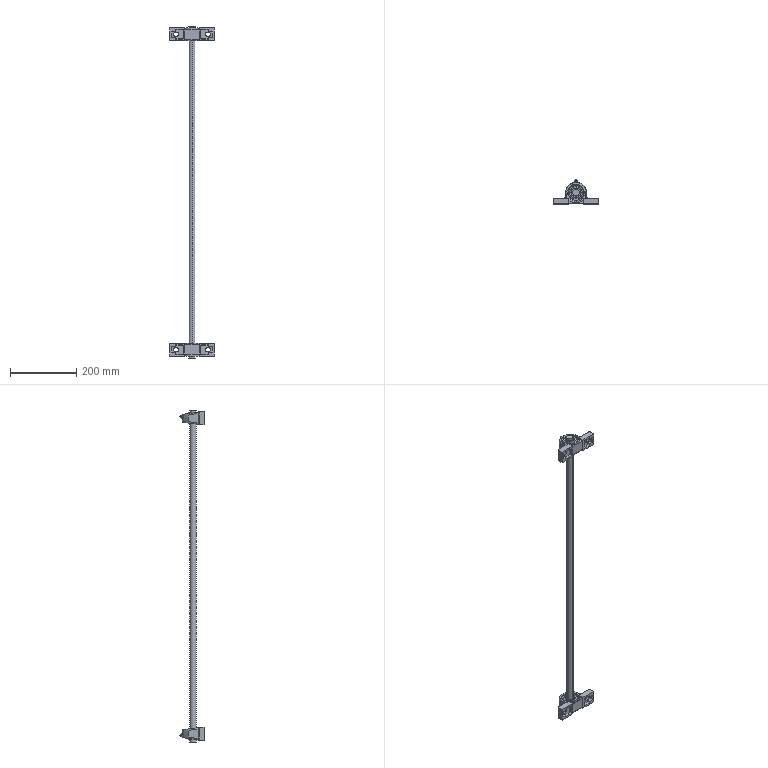Part | SolidWorks | 3 solids | 316 faces | box 134 x 72.66 x 1000 mm | volume 523004 mm3 | plane 114 | cylinder 88 | sphere 56 | cone 32 | torus 16 | spline 10 | commonest cylinder face diameters 2 x12 6 x12 27.83 x12 37.32 x12 51.695 x12 5.134 x8